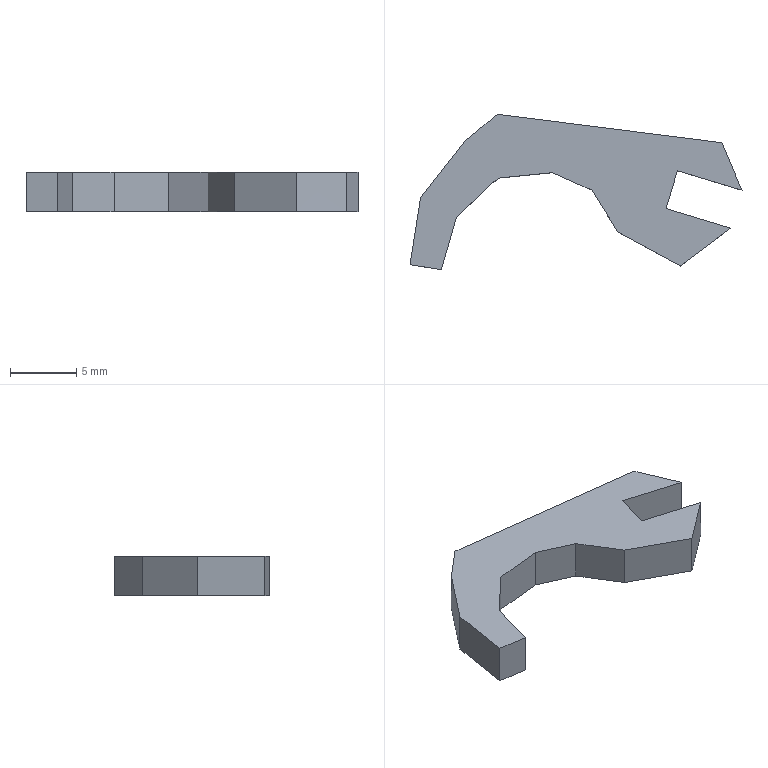Part | SolidWorks | features BaseBody 1 | 1 solid | 18 faces | box 25.116 x 11.758 x 3 mm | volume 409.356 mm3 | spline 12 | plane 6
STEP:
#1=CARTESIAN_POINT('',(49.749,1.825,-1.5));
#2=VERTEX_POINT('',#1);
#3=CARTESIAN_POINT('',(32.749,3.974,-1.5));
#4=VERTEX_POINT('',#3);
#5=CARTESIAN_POINT('',(49.749,1.825,-1.5));
#6=CARTESIAN_POINT('',(44.082,2.541,-1.5));
#7=CARTESIAN_POINT('',(38.416,3.258,-1.5));
#8=CARTESIAN_POINT('',(32.749,3.974,-1.5));
#9=B_SPLINE_CURVE_WITH_KNOTS('',3,(#5,#6,#7,#8),.UNSPECIFIED.,.F.,.F.,(4,4),(0.913,1.),.UNSPECIFIED.);
#10=EDGE_CURVE('',#2,#4,#9,.T.);
#11=ORIENTED_EDGE('',*,*,#10,.F.);
#12=CARTESIAN_POINT('',(51.278,-1.768,-1.5));
#13=VERTEX_POINT('',#12);
#14=CARTESIAN_POINT('',(51.278,-1.768,-1.5));
#15=DIRECTION('',(-0.3915,0.9202,0.));
#16=VECTOR('',#15,1000.);
#17=LINE('',#14,#16);
#18=EDGE_CURVE('',#13,#2,#17,.T.);
#19=ORIENTED_EDGE('',*,*,#18,.F.);
#20=CARTESIAN_POINT('',(46.394,-0.2969,-1.5));
#21=VERTEX_POINT('',#20);
#22=CARTESIAN_POINT('',(46.394,-0.2969,-1.5));
#23=DIRECTION('',(0.9575,-0.2885,0.));
#24=VECTOR('',#23,1000.);
#25=LINE('',#22,#24);
#26=EDGE_CURVE('',#21,#13,#25,.T.);
#27=ORIENTED_EDGE('',*,*,#26,.F.);
#28=CARTESIAN_POINT('',(45.529,-3.169,-1.5));
#29=VERTEX_POINT('',#28);
#30=CARTESIAN_POINT('',(45.529,-3.169,-1.5));
#31=DIRECTION('',(0.2885,0.9575,0.));
#32=VECTOR('',#31,1000.);
#33=LINE('',#30,#32);
#34=EDGE_CURVE('',#29,#21,#33,.T.);
#35=ORIENTED_EDGE('',*,*,#34,.F.);
#36=CARTESIAN_POINT('',(50.412,-4.641,-1.5));
#37=VERTEX_POINT('',#36);
#38=CARTESIAN_POINT('',(45.529,-3.169,-1.5));
#39=DIRECTION('',(-0.9575,0.2885,0.));
#40=VECTOR('',#39,1000.);
#41=LINE('',#38,#40);
#42=EDGE_CURVE('',#37,#29,#41,.T.);
#43=ORIENTED_EDGE('',*,*,#42,.F.);
#44=CARTESIAN_POINT('',(46.616,-7.504,-1.5));
#45=VERTEX_POINT('',#44);
#46=CARTESIAN_POINT('',(46.616,-7.504,-1.5));
#47=CARTESIAN_POINT('',(47.881,-6.548,-1.5));
#48=CARTESIAN_POINT('',(50.412,-4.641,-1.5));
#49=B_SPLINE_CURVE_WITH_KNOTS('',2,(#46,#47,#48),.UNSPECIFIED.,.F.,.F.,(3,3),(0.4348,0.4783),.UNSPECIFIED.);
#50=EDGE_CURVE('',#45,#37,#49,.T.);
#51=ORIENTED_EDGE('',*,*,#50,.F.);
#52=CARTESIAN_POINT('',(41.909,-4.958,-1.5));
#53=VERTEX_POINT('',#52);
#54=CARTESIAN_POINT('',(41.909,-4.958,-1.5));
#55=CARTESIAN_POINT('',(43.477,-5.807,-1.5));
#56=CARTESIAN_POINT('',(45.047,-6.655,-1.5));
#57=CARTESIAN_POINT('',(46.616,-7.504,-1.5));
#58=B_SPLINE_CURVE_WITH_KNOTS('',3,(#54,#55,#56,#57),.UNSPECIFIED.,.F.,.F.,(4,4),(0.3913,0.4348),.UNSPECIFIED.);
#59=EDGE_CURVE('',#53,#45,#58,.T.);
#60=ORIENTED_EDGE('',*,*,#59,.F.);
#61=CARTESIAN_POINT('',(39.937,-1.783,-1.5));
#62=VERTEX_POINT('',#61);
#63=CARTESIAN_POINT('',(39.937,-1.783,-1.5));
#64=CARTESIAN_POINT('',(40.594,-2.84,-1.5));
#65=CARTESIAN_POINT('',(41.252,-3.899,-1.5));
#66=CARTESIAN_POINT('',(41.909,-4.958,-1.5));
#67=B_SPLINE_CURVE_WITH_KNOTS('',3,(#63,#64,#65,#66),.UNSPECIFIED.,.F.,.F.,(4,4),(0.3478,0.3913),.UNSPECIFIED.);
#68=EDGE_CURVE('',#62,#53,#67,.T.);
#69=ORIENTED_EDGE('',*,*,#68,.F.);
#70=CARTESIAN_POINT('',(36.95,-0.4427,-1.5));
#71=VERTEX_POINT('',#70);
#72=CARTESIAN_POINT('',(36.95,-0.4427,-1.5));
#73=CARTESIAN_POINT('',(37.947,-0.8896,-1.5));
#74=CARTESIAN_POINT('',(38.941,-1.336,-1.5));
#75=CARTESIAN_POINT('',(39.937,-1.783,-1.5));
#76=B_SPLINE_CURVE_WITH_KNOTS('',3,(#72,#73,#74,#75),.UNSPECIFIED.,.F.,.F.,(4,4),(0.3043,0.3478),.UNSPECIFIED.);
#77=EDGE_CURVE('',#71,#62,#76,.T.);
#78=ORIENTED_EDGE('',*,*,#77,.F.);
#79=CARTESIAN_POINT('',(32.823,-0.8567,-1.5));
#80=VERTEX_POINT('',#79);
#81=CARTESIAN_POINT('',(32.823,-0.8567,-1.5));
#82=CARTESIAN_POINT('',(34.201,-0.7197,-1.5));
#83=CARTESIAN_POINT('',(35.575,-0.5811,-1.5));
#84=CARTESIAN_POINT('',(36.95,-0.4427,-1.5));
#85=B_SPLINE_CURVE_WITH_KNOTS('',3,(#81,#82,#83,#84),.UNSPECIFIED.,.F.,.F.,(4,4),(0.2609,0.3043),.UNSPECIFIED.);
#86=EDGE_CURVE('',#80,#71,#85,.T.);
#87=ORIENTED_EDGE('',*,*,#86,.F.);
#88=CARTESIAN_POINT('',(29.674,-3.825,-1.5));
#89=VERTEX_POINT('',#88);
#90=CARTESIAN_POINT('',(29.674,-3.825,-1.5));
#91=CARTESIAN_POINT('',(30.724,-2.835,-1.5));
#92=CARTESIAN_POINT('',(31.775,-1.846,-1.5));
#93=CARTESIAN_POINT('',(32.823,-0.8567,-1.5));
#94=B_SPLINE_CURVE_WITH_KNOTS('',3,(#90,#91,#92,#93),.UNSPECIFIED.,.F.,.F.,(4,4),(0.2174,0.2609),.UNSPECIFIED.);
#95=EDGE_CURVE('',#89,#80,#94,.T.);
#96=ORIENTED_EDGE('',*,*,#95,.F.);
#97=CARTESIAN_POINT('',(28.532,-7.783,-1.5));
#98=VERTEX_POINT('',#97);
#99=CARTESIAN_POINT('',(28.532,-7.783,-1.5));
#100=CARTESIAN_POINT('',(28.913,-6.463,-1.5));
#101=CARTESIAN_POINT('',(29.293,-5.143,-1.5));
#102=CARTESIAN_POINT('',(29.674,-3.825,-1.5));
#103=B_SPLINE_CURVE_WITH_KNOTS('',3,(#99,#100,#101,#102),.UNSPECIFIED.,.F.,.F.,(4,4),(0.1739,0.2174),.UNSPECIFIED.);
#104=EDGE_CURVE('',#98,#89,#103,.T.);
#105=ORIENTED_EDGE('',*,*,#104,.F.);
#106=CARTESIAN_POINT('',(26.162,-7.411,-1.5));
#107=VERTEX_POINT('',#106);
#108=CARTESIAN_POINT('',(26.162,-7.411,-1.5));
#109=CARTESIAN_POINT('',(26.952,-7.534,-1.5));
#110=CARTESIAN_POINT('',(27.742,-7.659,-1.5));
#111=CARTESIAN_POINT('',(28.532,-7.783,-1.5));
#112=B_SPLINE_CURVE_WITH_KNOTS('',3,(#108,#109,#110,#111),.UNSPECIFIED.,.F.,.F.,(4,4),(0.1304,0.1739),.UNSPECIFIED.);
#113=EDGE_CURVE('',#107,#98,#112,.T.);
#114=ORIENTED_EDGE('',*,*,#113,.F.);
#115=CARTESIAN_POINT('',(26.966,-2.331,-1.5));
#116=VERTEX_POINT('',#115);
#117=CARTESIAN_POINT('',(26.966,-2.331,-1.5));
#118=CARTESIAN_POINT('',(26.696,-4.024,-1.5));
#119=CARTESIAN_POINT('',(26.428,-5.716,-1.5));
#120=CARTESIAN_POINT('',(26.162,-7.411,-1.5));
#121=B_SPLINE_CURVE_WITH_KNOTS('',3,(#117,#118,#119,#120),.UNSPECIFIED.,.F.,.F.,(4,4),(0.08696,0.1304),.UNSPECIFIED.);
#122=EDGE_CURVE('',#116,#107,#121,.T.);
#123=ORIENTED_EDGE('',*,*,#122,.F.);
#124=CARTESIAN_POINT('',(30.236,1.845,-1.5));
#125=VERTEX_POINT('',#124);
#126=CARTESIAN_POINT('',(30.236,1.845,-1.5));
#127=CARTESIAN_POINT('',(29.145,0.4517,-1.5));
#128=CARTESIAN_POINT('',(28.055,-0.9382,-1.5));
#129=CARTESIAN_POINT('',(26.966,-2.331,-1.5));
#130=B_SPLINE_CURVE_WITH_KNOTS('',3,(#126,#127,#128,#129),.UNSPECIFIED.,.F.,.F.,(4,4),(0.04348,0.08696),.UNSPECIFIED.);
#131=EDGE_CURVE('',#125,#116,#130,.T.);
#132=ORIENTED_EDGE('',*,*,#131,.F.);
#133=CARTESIAN_POINT('',(32.749,3.974,-1.5));
#134=CARTESIAN_POINT('',(31.912,3.263,-1.5));
#135=CARTESIAN_POINT('',(31.073,2.553,-1.5));
#136=CARTESIAN_POINT('',(30.236,1.845,-1.5));
#137=B_SPLINE_CURVE_WITH_KNOTS('',3,(#133,#134,#135,#136),.UNSPECIFIED.,.F.,.F.,(4,4),(0.,0.04348),.UNSPECIFIED.);
#138=EDGE_CURVE('',#4,#125,#137,.T.);
#139=ORIENTED_EDGE('',*,*,#138,.F.);
#140=EDGE_LOOP('',(#11,#19,#27,#35,#43,#51,#60,#69,#78,#87,#96,#105,#114,#123,#132,#139));
#141=FACE_OUTER_BOUND('',#140,.T.);
#142=CARTESIAN_POINT('',(41.249,2.9,-1.5));
#143=DIRECTION('',(0.,0.,1.));
#144=DIRECTION('',(1.,0.,0.));
#145=AXIS2_PLACEMENT_3D('',#142,#143,#144);
#146=PLANE('',#145);
#147=ADVANCED_FACE('',(#141),#146,.F.);
#148=CARTESIAN_POINT('',(49.749,1.825,1.5));
#149=VERTEX_POINT('',#148);
#150=CARTESIAN_POINT('',(32.749,3.974,1.5));
#151=VERTEX_POINT('',#150);
#152=CARTESIAN_POINT('',(49.749,1.825,1.5));
#153=CARTESIAN_POINT('',(44.082,2.541,1.5));
#154=CARTESIAN_POINT('',(38.416,3.258,1.5));
#155=CARTESIAN_POINT('',(32.749,3.974,1.5));
#156=B_SPLINE_CURVE_WITH_KNOTS('',3,(#152,#153,#154,#155),.UNSPECIFIED.,.F.,.F.,(4,4),(0.913,1.),.UNSPECIFIED.);
#157=EDGE_CURVE('',#149,#151,#156,.T.);
#158=ORIENTED_EDGE('',*,*,#157,.T.);
#159=CARTESIAN_POINT('',(30.236,1.845,1.5));
#160=VERTEX_POINT('',#159);
#161=CARTESIAN_POINT('',(32.749,3.974,1.5));
#162=CARTESIAN_POINT('',(31.912,3.263,1.5));
#163=CARTESIAN_POINT('',(31.073,2.553,1.5));
#164=CARTESIAN_POINT('',(30.236,1.845,1.5));
#165=B_SPLINE_CURVE_WITH_KNOTS('',3,(#161,#162,#163,#164),.UNSPECIFIED.,.F.,.F.,(4,4),(0.,0.04348),.UNSPECIFIED.);
#166=EDGE_CURVE('',#151,#160,#165,.T.);
#167=ORIENTED_EDGE('',*,*,#166,.T.);
#168=CARTESIAN_POINT('',(26.966,-2.331,1.5));
#169=VERTEX_POINT('',#168);
#170=CARTESIAN_POINT('',(30.236,1.845,1.5));
#171=CARTESIAN_POINT('',(29.145,0.4517,1.5));
#172=CARTESIAN_POINT('',(28.055,-0.9382,1.5));
#173=CARTESIAN_POINT('',(26.966,-2.331,1.5));
#174=B_SPLINE_CURVE_WITH_KNOTS('',3,(#170,#171,#172,#173),.UNSPECIFIED.,.F.,.F.,(4,4),(0.04348,0.08696),.UNSPECIFIED.);
#175=EDGE_CURVE('',#160,#169,#174,.T.);
#176=ORIENTED_EDGE('',*,*,#175,.T.);
#177=CARTESIAN_POINT('',(26.162,-7.411,1.5));
#178=VERTEX_POINT('',#177);
#179=CARTESIAN_POINT('',(26.966,-2.331,1.5));
#180=CARTESIAN_POINT('',(26.696,-4.024,1.5));
#181=CARTESIAN_POINT('',(26.428,-5.716,1.5));
#182=CARTESIAN_POINT('',(26.162,-7.411,1.5));
#183=B_SPLINE_CURVE_WITH_KNOTS('',3,(#179,#180,#181,#182),.UNSPECIFIED.,.F.,.F.,(4,4),(0.08696,0.1304),.UNSPECIFIED.);
#184=EDGE_CURVE('',#169,#178,#183,.T.);
#185=ORIENTED_EDGE('',*,*,#184,.T.);
#186=CARTESIAN_POINT('',(28.532,-7.783,1.5));
#187=VERTEX_POINT('',#186);
#188=CARTESIAN_POINT('',(26.162,-7.411,1.5));
#189=CARTESIAN_POINT('',(26.952,-7.534,1.5));
#190=CARTESIAN_POINT('',(27.742,-7.659,1.5));
#191=CARTESIAN_POINT('',(28.532,-7.783,1.5));
#192=B_SPLINE_CURVE_WITH_KNOTS('',3,(#188,#189,#190,#191),.UNSPECIFIED.,.F.,.F.,(4,4),(0.1304,0.1739),.UNSPECIFIED.);
#193=EDGE_CURVE('',#178,#187,#192,.T.);
#194=ORIENTED_EDGE('',*,*,#193,.T.);
#195=CARTESIAN_POINT('',(29.674,-3.825,1.5));
#196=VERTEX_POINT('',#195);
#197=CARTESIAN_POINT('',(28.532,-7.783,1.5));
#198=CARTESIAN_POINT('',(28.913,-6.463,1.5));
#199=CARTESIAN_POINT('',(29.293,-5.143,1.5));
#200=CARTESIAN_POINT('',(29.674,-3.825,1.5));
#201=B_SPLINE_CURVE_WITH_KNOTS('',3,(#197,#198,#199,#200),.UNSPECIFIED.,.F.,.F.,(4,4),(0.1739,0.2174),.UNSPECIFIED.);
#202=EDGE_CURVE('',#187,#196,#201,.T.);
#203=ORIENTED_EDGE('',*,*,#202,.T.);
#204=CARTESIAN_POINT('',(32.823,-0.8567,1.5));
#205=VERTEX_POINT('',#204);
#206=CARTESIAN_POINT('',(29.674,-3.825,1.5));
#207=CARTESIAN_POINT('',(30.724,-2.835,1.5));
#208=CARTESIAN_POINT('',(31.775,-1.846,1.5));
#209=CARTESIAN_POINT('',(32.823,-0.8567,1.5));
#210=B_SPLINE_CURVE_WITH_KNOTS('',3,(#206,#207,#208,#209),.UNSPECIFIED.,.F.,.F.,(4,4),(0.2174,0.2609),.UNSPECIFIED.);
#211=EDGE_CURVE('',#196,#205,#210,.T.);
#212=ORIENTED_EDGE('',*,*,#211,.T.);
#213=CARTESIAN_POINT('',(36.95,-0.4427,1.5));
#214=VERTEX_POINT('',#213);
#215=CARTESIAN_POINT('',(32.823,-0.8567,1.5));
#216=CARTESIAN_POINT('',(34.201,-0.7197,1.5));
#217=CARTESIAN_POINT('',(35.575,-0.5811,1.5));
#218=CARTESIAN_POINT('',(36.95,-0.4427,1.5));
#219=B_SPLINE_CURVE_WITH_KNOTS('',3,(#215,#216,#217,#218),.UNSPECIFIED.,.F.,.F.,(4,4),(0.2609,0.3043),.UNSPECIFIED.);
#220=EDGE_CURVE('',#205,#214,#219,.T.);
#221=ORIENTED_EDGE('',*,*,#220,.T.);
#222=CARTESIAN_POINT('',(39.937,-1.783,1.5));
#223=VERTEX_POINT('',#222);
#224=CARTESIAN_POINT('',(36.95,-0.4427,1.5));
#225=CARTESIAN_POINT('',(37.947,-0.8896,1.5));
#226=CARTESIAN_POINT('',(38.941,-1.336,1.5));
#227=CARTESIAN_POINT('',(39.937,-1.783,1.5));
#228=B_SPLINE_CURVE_WITH_KNOTS('',3,(#224,#225,#226,#227),.UNSPECIFIED.,.F.,.F.,(4,4),(0.3043,0.3478),.UNSPECIFIED.);
#229=EDGE_CURVE('',#214,#223,#228,.T.);
#230=ORIENTED_EDGE('',*,*,#229,.T.);
#231=CARTESIAN_POINT('',(41.909,-4.958,1.5));
#232=VERTEX_POINT('',#231);
#233=CARTESIAN_POINT('',(39.937,-1.783,1.5));
#234=CARTESIAN_POINT('',(40.594,-2.84,1.5));
#235=CARTESIAN_POINT('',(41.252,-3.899,1.5));
#236=CARTESIAN_POINT('',(41.909,-4.958,1.5));
#237=B_SPLINE_CURVE_WITH_KNOTS('',3,(#233,#234,#235,#236),.UNSPECIFIED.,.F.,.F.,(4,4),(0.3478,0.3913),.UNSPECIFIED.);
#238=EDGE_CURVE('',#223,#232,#237,.T.);
#239=ORIENTED_EDGE('',*,*,#238,.T.);
#240=CARTESIAN_POINT('',(46.616,-7.504,1.5));
#241=VERTEX_POINT('',#240);
#242=CARTESIAN_POINT('',(41.909,-4.958,1.5));
#243=CARTESIAN_POINT('',(43.477,-5.807,1.5));
#244=CARTESIAN_POINT('',(45.047,-6.655,1.5));
#245=CARTESIAN_POINT('',(46.616,-7.504,1.5));
#246=B_SPLINE_CURVE_WITH_KNOTS('',3,(#242,#243,#244,#245),.UNSPECIFIED.,.F.,.F.,(4,4),(0.3913,0.4348),.UNSPECIFIED.);
#247=EDGE_CURVE('',#232,#241,#246,.T.);
#248=ORIENTED_EDGE('',*,*,#247,.T.);
#249=CARTESIAN_POINT('',(50.412,-4.641,1.5));
#250=VERTEX_POINT('',#249);
#251=CARTESIAN_POINT('',(46.616,-7.504,1.5));
#252=CARTESIAN_POINT('',(47.881,-6.548,1.5));
#253=CARTESIAN_POINT('',(50.412,-4.641,1.5));
#254=B_SPLINE_CURVE_WITH_KNOTS('',2,(#251,#252,#253),.UNSPECIFIED.,.F.,.F.,(3,3),(0.4348,0.4783),.UNSPECIFIED.);
#255=EDGE_CURVE('',#241,#250,#254,.T.);
#256=ORIENTED_EDGE('',*,*,#255,.T.);
#257=CARTESIAN_POINT('',(45.529,-3.169,1.5));
#258=VERTEX_POINT('',#257);
#259=CARTESIAN_POINT('',(45.529,-3.169,1.5));
#260=DIRECTION('',(-0.9575,0.2885,0.));
#261=VECTOR('',#260,1000.);
#262=LINE('',#259,#261);
#263=EDGE_CURVE('',#250,#258,#262,.T.);
#264=ORIENTED_EDGE('',*,*,#263,.T.);
#265=CARTESIAN_POINT('',(46.394,-0.2969,1.5));
#266=VERTEX_POINT('',#265);
#267=CARTESIAN_POINT('',(45.529,-3.169,1.5));
#268=DIRECTION('',(0.2885,0.9575,0.));
#269=VECTOR('',#268,1000.);
#270=LINE('',#267,#269);
#271=EDGE_CURVE('',#258,#266,#270,.T.);
#272=ORIENTED_EDGE('',*,*,#271,.T.);
#273=CARTESIAN_POINT('',(51.278,-1.768,1.5));
#274=VERTEX_POINT('',#273);
#275=CARTESIAN_POINT('',(46.394,-0.2969,1.5));
#276=DIRECTION('',(0.9575,-0.2885,0.));
#277=VECTOR('',#276,1000.);
#278=LINE('',#275,#277);
#279=EDGE_CURVE('',#266,#274,#278,.T.);
#280=ORIENTED_EDGE('',*,*,#279,.T.);
#281=CARTESIAN_POINT('',(51.278,-1.768,1.5));
#282=DIRECTION('',(-0.3915,0.9202,0.));
#283=VECTOR('',#282,1000.);
#284=LINE('',#281,#283);
#285=EDGE_CURVE('',#274,#149,#284,.T.);
#286=ORIENTED_EDGE('',*,*,#285,.T.);
#287=EDGE_LOOP('',(#158,#167,#176,#185,#194,#203,#212,#221,#230,#239,#248,#256,#264,#272,#280,#286));
#288=FACE_OUTER_BOUND('',#287,.T.);
#289=CARTESIAN_POINT('',(41.249,2.9,1.5));
#290=DIRECTION('',(0.,0.,1.));
#291=DIRECTION('',(1.,0.,0.));
#292=AXIS2_PLACEMENT_3D('',#289,#290,#291);
#293=PLANE('',#292);
#294=ADVANCED_FACE('',(#288),#293,.T.);
#295=ORIENTED_EDGE('',*,*,#18,.T.);
#296=CARTESIAN_POINT('',(49.749,1.825,1.5));
#297=DIRECTION('',(0.,0.,-1.));
#298=VECTOR('',#297,1000.);
#299=LINE('',#296,#298);
#300=EDGE_CURVE('',#149,#2,#299,.T.);
#301=ORIENTED_EDGE('',*,*,#300,.F.);
#302=ORIENTED_EDGE('',*,*,#285,.F.);
#303=CARTESIAN_POINT('',(51.278,-1.768,1.5));
#304=DIRECTION('',(0.,0.,-1.));
#305=VECTOR('',#304,1000.);
#306=LINE('',#303,#305);
#307=EDGE_CURVE('',#274,#13,#306,.T.);
#308=ORIENTED_EDGE('',*,*,#307,.T.);
#309=EDGE_LOOP('',(#295,#301,#302,#308));
#310=FACE_OUTER_BOUND('',#309,.T.);
#311=CARTESIAN_POINT('',(51.278,-1.768,1.5));
#312=DIRECTION('',(-0.9202,-0.3915,0.));
#313=DIRECTION('',(-0.3915,0.9202,0.));
#314=AXIS2_PLACEMENT_3D('',#311,#312,#313);
#315=PLANE('',#314);
#316=ADVANCED_FACE('',(#310),#315,.F.);
#317=ORIENTED_EDGE('',*,*,#26,.T.);
#318=ORIENTED_EDGE('',*,*,#307,.F.);
#319=ORIENTED_EDGE('',*,*,#279,.F.);
#320=CARTESIAN_POINT('',(46.394,-0.2969,1.5));
#321=DIRECTION('',(0.,0.,-1.));
#322=VECTOR('',#321,1000.);
#323=LINE('',#320,#322);
#324=EDGE_CURVE('',#266,#21,#323,.T.);
#325=ORIENTED_EDGE('',*,*,#324,.T.);
#326=EDGE_LOOP('',(#317,#318,#319,#325));
#327=FACE_OUTER_BOUND('',#326,.T.);
#328=CARTESIAN_POINT('',(46.394,-0.2969,1.5));
#329=DIRECTION('',(0.2885,0.9575,0.));
#330=DIRECTION('',(0.,0.,-1.));
#331=AXIS2_PLACEMENT_3D('',#328,#329,#330);
#332=PLANE('',#331);
#333=ADVANCED_FACE('',(#327),#332,.F.);
#334=ORIENTED_EDGE('',*,*,#34,.T.);
#335=ORIENTED_EDGE('',*,*,#324,.F.);
#336=ORIENTED_EDGE('',*,*,#271,.F.);
#337=CARTESIAN_POINT('',(45.529,-3.169,1.5));
#338=DIRECTION('',(0.,0.,-1.));
#339=VECTOR('',#338,1000.);
#340=LINE('',#337,#339);
#341=EDGE_CURVE('',#258,#29,#340,.T.);
#342=ORIENTED_EDGE('',*,*,#341,.T.);
#343=EDGE_LOOP('',(#334,#335,#336,#342));
#344=FACE_OUTER_BOUND('',#343,.T.);
#345=CARTESIAN_POINT('',(45.529,-3.169,1.5));
#346=DIRECTION('',(-0.9575,0.2885,0.));
#347=DIRECTION('',(0.,0.,1.));
#348=AXIS2_PLACEMENT_3D('',#345,#346,#347);
#349=PLANE('',#348);
#350=ADVANCED_FACE('',(#344),#349,.F.);
#351=ORIENTED_EDGE('',*,*,#42,.T.);
#352=ORIENTED_EDGE('',*,*,#341,.F.);
#353=ORIENTED_EDGE('',*,*,#263,.F.);
#354=CARTESIAN_POINT('',(50.412,-4.641,1.5));
#355=DIRECTION('',(0.,0.,-1.));
#356=VECTOR('',#355,1000.);
#357=LINE('',#354,#356);
#358=EDGE_CURVE('',#250,#37,#357,.T.);
#359=ORIENTED_EDGE('',*,*,#358,.T.);
#360=EDGE_LOOP('',(#351,#352,#353,#359));
#361=FACE_OUTER_BOUND('',#360,.T.);
#362=CARTESIAN_POINT('',(45.529,-3.169,1.5));
#363=DIRECTION('',(-0.2885,-0.9575,0.));
#364=DIRECTION('',(-0.9575,0.2885,0.));
#365=AXIS2_PLACEMENT_3D('',#362,#363,#364);
#366=PLANE('',#365);
#367=ADVANCED_FACE('',(#361),#366,.F.);
#368=ORIENTED_EDGE('',*,*,#50,.T.);
#369=ORIENTED_EDGE('',*,*,#358,.F.);
#370=ORIENTED_EDGE('',*,*,#255,.F.);
#371=CARTESIAN_POINT('',(46.616,-7.504,1.5));
#372=DIRECTION('',(0.,0.,-1.));
#373=VECTOR('',#372,1000.);
#374=LINE('',#371,#373);
#375=EDGE_CURVE('',#241,#45,#374,.T.);
#376=ORIENTED_EDGE('',*,*,#375,.T.);
#377=EDGE_LOOP('',(#368,#369,#370,#376));
#378=FACE_OUTER_BOUND('',#377,.T.);
#379=CARTESIAN_POINT('',(46.616,-7.504,1.5));
#380=CARTESIAN_POINT('',(46.616,-7.504,-1.5));
#381=CARTESIAN_POINT('',(47.881,-6.548,1.5));
#382=CARTESIAN_POINT('',(47.881,-6.548,-1.5));
#383=CARTESIAN_POINT('',(50.412,-4.641,1.5));
#384=CARTESIAN_POINT('',(50.412,-4.641,-1.5));
#385=B_SPLINE_SURFACE_WITH_KNOTS('',2,1,((#379,#380),(#381,#382),(#383,#384)),.UNSPECIFIED.,.F.,.F.,.F.,(3,3),(2,2),(0.4348,0.4783),(0.,1.),.UNSPECIFIED.);
#386=ADVANCED_FACE('',(#378),#385,.F.);
#387=ORIENTED_EDGE('',*,*,#59,.T.);
#388=ORIENTED_EDGE('',*,*,#375,.F.);
#389=ORIENTED_EDGE('',*,*,#247,.F.);
#390=CARTESIAN_POINT('',(41.909,-4.958,1.5));
#391=DIRECTION('',(0.,0.,-1.));
#392=VECTOR('',#391,1000.);
#393=LINE('',#390,#392);
#394=EDGE_CURVE('',#232,#53,#393,.T.);
#395=ORIENTED_EDGE('',*,*,#394,.T.);
#396=EDGE_LOOP('',(#387,#388,#389,#395));
#397=FACE_OUTER_BOUND('',#396,.T.);
#398=CARTESIAN_POINT('',(41.909,-4.958,1.5));
#399=CARTESIAN_POINT('',(41.909,-4.958,-1.5));
#400=CARTESIAN_POINT('',(43.477,-5.807,1.5));
#401=CARTESIAN_POINT('',(43.477,-5.807,-1.5));
#402=CARTESIAN_POINT('',(45.047,-6.655,1.5));
#403=CARTESIAN_POINT('',(45.047,-6.655,-1.5));
#404=CARTESIAN_POINT('',(46.616,-7.504,1.5));
#405=CARTESIAN_POINT('',(46.616,-7.504,-1.5));
#406=B_SPLINE_SURFACE_WITH_KNOTS('',3,1,((#398,#399),(#400,#401),(#402,#403),(#404,#405)),.UNSPECIFIED.,.F.,.F.,.F.,(4,4),(2,2),(0.3913,0.4348),(0.,1.),.UNSPECIFIED.);
#407=ADVANCED_FACE('',(#397),#406,.F.);
#408=ORIENTED_EDGE('',*,*,#68,.T.);
#409=ORIENTED_EDGE('',*,*,#394,.F.);
#410=ORIENTED_EDGE('',*,*,#238,.F.);
#411=CARTESIAN_POINT('',(39.937,-1.783,1.5));
#412=DIRECTION('',(0.,0.,-1.));
#413=VECTOR('',#412,1000.);
#414=LINE('',#411,#413);
#415=EDGE_CURVE('',#223,#62,#414,.T.);
#416=ORIENTED_EDGE('',*,*,#415,.T.);
#417=EDGE_LOOP('',(#408,#409,#410,#416));
#418=FACE_OUTER_BOUND('',#417,.T.);
#419=CARTESIAN_POINT('',(39.937,-1.783,1.5));
#420=CARTESIAN_POINT('',(39.937,-1.783,-1.5));
#421=CARTESIAN_POINT('',(40.594,-2.84,1.5));
#422=CARTESIAN_POINT('',(40.594,-2.84,-1.5));
#423=CARTESIAN_POINT('',(41.252,-3.899,1.5));
#424=CARTESIAN_POINT('',(41.252,-3.899,-1.5));
#425=CARTESIAN_POINT('',(41.909,-4.958,1.5));
#426=CARTESIAN_POINT('',(41.909,-4.958,-1.5));
#427=B_SPLINE_SURFACE_WITH_KNOTS('',3,1,((#419,#420),(#421,#422),(#423,#424),(#425,#426)),.UNSPECIFIED.,.F.,.F.,.F.,(4,4),(2,2),(0.3478,0.3913),(0.,1.),.UNSPECIFIED.);
#428=ADVANCED_FACE('',(#418),#427,.F.);
#429=ORIENTED_EDGE('',*,*,#77,.T.);
#430=ORIENTED_EDGE('',*,*,#415,.F.);
#431=ORIENTED_EDGE('',*,*,#229,.F.);
#432=CARTESIAN_POINT('',(36.95,-0.4427,1.5));
#433=DIRECTION('',(0.,0.,-1.));
#434=VECTOR('',#433,1000.);
#435=LINE('',#432,#434);
#436=EDGE_CURVE('',#214,#71,#435,.T.);
#437=ORIENTED_EDGE('',*,*,#436,.T.);
#438=EDGE_LOOP('',(#429,#430,#431,#437));
#439=FACE_OUTER_BOUND('',#438,.T.);
#440=CARTESIAN_POINT('',(36.95,-0.4427,1.5));
#441=CARTESIAN_POINT('',(36.95,-0.4427,-1.5));
#442=CARTESIAN_POINT('',(37.947,-0.8896,1.5));
#443=CARTESIAN_POINT('',(37.947,-0.8896,-1.5));
#444=CARTESIAN_POINT('',(38.941,-1.336,1.5));
#445=CARTESIAN_POINT('',(38.941,-1.336,-1.5));
#446=CARTESIAN_POINT('',(39.937,-1.783,1.5));
#447=CARTESIAN_POINT('',(39.937,-1.783,-1.5));
#448=B_SPLINE_SURFACE_WITH_KNOTS('',3,1,((#440,#441),(#442,#443),(#444,#445),(#446,#447)),.UNSPECIFIED.,.F.,.F.,.F.,(4,4),(2,2),(0.3043,0.3478),(0.,1.),.UNSPECIFIED.);
#449=ADVANCED_FACE('',(#439),#448,.F.);
#450=ORIENTED_EDGE('',*,*,#86,.T.);
#451=ORIENTED_EDGE('',*,*,#436,.F.);
#452=ORIENTED_EDGE('',*,*,#220,.F.);
#453=CARTESIAN_POINT('',(32.823,-0.8567,1.5));
#454=DIRECTION('',(0.,0.,-1.));
#455=VECTOR('',#454,1000.);
#456=LINE('',#453,#455);
#457=EDGE_CURVE('',#205,#80,#456,.T.);
#458=ORIENTED_EDGE('',*,*,#457,.T.);
#459=EDGE_LOOP('',(#450,#451,#452,#458));
#460=FACE_OUTER_BOUND('',#459,.T.);
#461=CARTESIAN_POINT('',(32.823,-0.8567,1.5));
#462=CARTESIAN_POINT('',(32.823,-0.8567,-1.5));
#463=CARTESIAN_POINT('',(34.201,-0.7197,1.5));
#464=CARTESIAN_POINT('',(34.201,-0.7197,-1.5));
#465=CARTESIAN_POINT('',(35.575,-0.5811,1.5));
#466=CARTESIAN_POINT('',(35.575,-0.5811,-1.5));
#467=CARTESIAN_POINT('',(36.95,-0.4427,1.5));
#468=CARTESIAN_POINT('',(36.95,-0.4427,-1.5));
#469=B_SPLINE_SURFACE_WITH_KNOTS('',3,1,((#461,#462),(#463,#464),(#465,#466),(#467,#468)),.UNSPECIFIED.,.F.,.F.,.F.,(4,4),(2,2),(0.2609,0.3043),(0.,1.),.UNSPECIFIED.);
#470=ADVANCED_FACE('',(#460),#469,.F.);
#471=ORIENTED_EDGE('',*,*,#95,.T.);
#472=ORIENTED_EDGE('',*,*,#457,.F.);
#473=ORIENTED_EDGE('',*,*,#211,.F.);
#474=CARTESIAN_POINT('',(29.674,-3.825,1.5));
#475=DIRECTION('',(0.,0.,-1.));
#476=VECTOR('',#475,1000.);
#477=LINE('',#474,#476);
#478=EDGE_CURVE('',#196,#89,#477,.T.);
#479=ORIENTED_EDGE('',*,*,#478,.T.);
#480=EDGE_LOOP('',(#471,#472,#473,#479));
#481=FACE_OUTER_BOUND('',#480,.T.);
#482=CARTESIAN_POINT('',(29.674,-3.825,1.5));
#483=CARTESIAN_POINT('',(29.674,-3.825,-1.5));
#484=CARTESIAN_POINT('',(30.724,-2.835,1.5));
#485=CARTESIAN_POINT('',(30.724,-2.835,-1.5));
#486=CARTESIAN_POINT('',(31.775,-1.846,1.5));
#487=CARTESIAN_POINT('',(31.775,-1.846,-1.5));
#488=CARTESIAN_POINT('',(32.823,-0.8567,1.5));
#489=CARTESIAN_POINT('',(32.823,-0.8567,-1.5));
#490=B_SPLINE_SURFACE_WITH_KNOTS('',3,1,((#482,#483),(#484,#485),(#486,#487),(#488,#489)),.UNSPECIFIED.,.F.,.F.,.F.,(4,4),(2,2),(0.2174,0.2609),(0.,1.),.UNSPECIFIED.);
#491=ADVANCED_FACE('',(#481),#490,.F.);
#492=ORIENTED_EDGE('',*,*,#104,.T.);
#493=ORIENTED_EDGE('',*,*,#478,.F.);
#494=ORIENTED_EDGE('',*,*,#202,.F.);
#495=CARTESIAN_POINT('',(28.532,-7.783,1.5));
#496=DIRECTION('',(0.,0.,-1.));
#497=VECTOR('',#496,1000.);
#498=LINE('',#495,#497);
#499=EDGE_CURVE('',#187,#98,#498,.T.);
#500=ORIENTED_EDGE('',*,*,#499,.T.);
#501=EDGE_LOOP('',(#492,#493,#494,#500));
#502=FACE_OUTER_BOUND('',#501,.T.);
#503=CARTESIAN_POINT('',(28.532,-7.783,1.5));
#504=CARTESIAN_POINT('',(28.532,-7.783,-1.5));
#505=CARTESIAN_POINT('',(28.913,-6.463,1.5));
#506=CARTESIAN_POINT('',(28.913,-6.463,-1.5));
#507=CARTESIAN_POINT('',(29.293,-5.143,1.5));
#508=CARTESIAN_POINT('',(29.293,-5.143,-1.5));
#509=CARTESIAN_POINT('',(29.674,-3.825,1.5));
#510=CARTESIAN_POINT('',(29.674,-3.825,-1.5));
#511=B_SPLINE_SURFACE_WITH_KNOTS('',3,1,((#503,#504),(#505,#506),(#507,#508),(#509,#510)),.UNSPECIFIED.,.F.,.F.,.F.,(4,4),(2,2),(0.1739,0.2174),(0.,1.),.UNSPECIFIED.);
#512=ADVANCED_FACE('',(#502),#511,.F.);
#513=ORIENTED_EDGE('',*,*,#113,.T.);
#514=ORIENTED_EDGE('',*,*,#499,.F.);
#515=ORIENTED_EDGE('',*,*,#193,.F.);
#516=CARTESIAN_POINT('',(26.162,-7.411,1.5));
#517=DIRECTION('',(0.,0.,-1.));
#518=VECTOR('',#517,1000.);
#519=LINE('',#516,#518);
#520=EDGE_CURVE('',#178,#107,#519,.T.);
#521=ORIENTED_EDGE('',*,*,#520,.T.);
#522=EDGE_LOOP('',(#513,#514,#515,#521));
#523=FACE_OUTER_BOUND('',#522,.T.);
#524=CARTESIAN_POINT('',(26.162,-7.411,1.5));
#525=CARTESIAN_POINT('',(26.162,-7.411,-1.5));
#526=CARTESIAN_POINT('',(26.952,-7.534,1.5));
#527=CARTESIAN_POINT('',(26.952,-7.534,-1.5));
#528=CARTESIAN_POINT('',(27.742,-7.659,1.5));
#529=CARTESIAN_POINT('',(27.742,-7.659,-1.5));
#530=CARTESIAN_POINT('',(28.532,-7.783,1.5));
#531=CARTESIAN_POINT('',(28.532,-7.783,-1.5));
#532=B_SPLINE_SURFACE_WITH_KNOTS('',3,1,((#524,#525),(#526,#527),(#528,#529),(#530,#531)),.UNSPECIFIED.,.F.,.F.,.F.,(4,4),(2,2),(0.1304,0.1739),(0.,1.),.UNSPECIFIED.);
#533=ADVANCED_FACE('',(#523),#532,.F.);
#534=ORIENTED_EDGE('',*,*,#122,.T.);
#535=ORIENTED_EDGE('',*,*,#520,.F.);
#536=ORIENTED_EDGE('',*,*,#184,.F.);
#537=CARTESIAN_POINT('',(26.966,-2.331,1.5));
#538=DIRECTION('',(0.,0.,-1.));
#539=VECTOR('',#538,1000.);
#540=LINE('',#537,#539);
#541=EDGE_CURVE('',#169,#116,#540,.T.);
#542=ORIENTED_EDGE('',*,*,#541,.T.);
#543=EDGE_LOOP('',(#534,#535,#536,#542));
#544=FACE_OUTER_BOUND('',#543,.T.);
#545=CARTESIAN_POINT('',(26.966,-2.331,1.5));
#546=CARTESIAN_POINT('',(26.966,-2.331,-1.5));
#547=CARTESIAN_POINT('',(26.696,-4.024,1.5));
#548=CARTESIAN_POINT('',(26.696,-4.024,-1.5));
#549=CARTESIAN_POINT('',(26.428,-5.716,1.5));
#550=CARTESIAN_POINT('',(26.428,-5.716,-1.5));
#551=CARTESIAN_POINT('',(26.162,-7.411,1.5));
#552=CARTESIAN_POINT('',(26.162,-7.411,-1.5));
#553=B_SPLINE_SURFACE_WITH_KNOTS('',3,1,((#545,#546),(#547,#548),(#549,#550),(#551,#552)),.UNSPECIFIED.,.F.,.F.,.F.,(4,4),(2,2),(0.08696,0.1304),(0.,1.),.UNSPECIFIED.);
#554=ADVANCED_FACE('',(#544),#553,.F.);
#555=ORIENTED_EDGE('',*,*,#131,.T.);
#556=ORIENTED_EDGE('',*,*,#541,.F.);
#557=ORIENTED_EDGE('',*,*,#175,.F.);
#558=CARTESIAN_POINT('',(30.236,1.845,1.5));
#559=DIRECTION('',(0.,0.,-1.));
#560=VECTOR('',#559,1000.);
#561=LINE('',#558,#560);
#562=EDGE_CURVE('',#160,#125,#561,.T.);
#563=ORIENTED_EDGE('',*,*,#562,.T.);
#564=EDGE_LOOP('',(#555,#556,#557,#563));
#565=FACE_OUTER_BOUND('',#564,.T.);
#566=CARTESIAN_POINT('',(30.236,1.845,1.5));
#567=CARTESIAN_POINT('',(30.236,1.845,-1.5));
#568=CARTESIAN_POINT('',(29.145,0.4517,1.5));
#569=CARTESIAN_POINT('',(29.145,0.4517,-1.5));
#570=CARTESIAN_POINT('',(28.055,-0.9382,1.5));
#571=CARTESIAN_POINT('',(28.055,-0.9382,-1.5));
#572=CARTESIAN_POINT('',(26.966,-2.331,1.5));
#573=CARTESIAN_POINT('',(26.966,-2.331,-1.5));
#574=B_SPLINE_SURFACE_WITH_KNOTS('',3,1,((#566,#567),(#568,#569),(#570,#571),(#572,#573)),.UNSPECIFIED.,.F.,.F.,.F.,(4,4),(2,2),(0.04348,0.08696),(0.,1.),.UNSPECIFIED.);
#575=ADVANCED_FACE('',(#565),#574,.F.);
#576=ORIENTED_EDGE('',*,*,#138,.T.);
#577=ORIENTED_EDGE('',*,*,#562,.F.);
#578=ORIENTED_EDGE('',*,*,#166,.F.);
#579=CARTESIAN_POINT('',(32.749,3.974,1.5));
#580=DIRECTION('',(0.,0.,-1.));
#581=VECTOR('',#580,1000.);
#582=LINE('',#579,#581);
#583=EDGE_CURVE('',#151,#4,#582,.T.);
#584=ORIENTED_EDGE('',*,*,#583,.T.);
#585=EDGE_LOOP('',(#576,#577,#578,#584));
#586=FACE_OUTER_BOUND('',#585,.T.);
#587=CARTESIAN_POINT('',(32.749,3.974,1.5));
#588=CARTESIAN_POINT('',(32.749,3.974,-1.5));
#589=CARTESIAN_POINT('',(31.912,3.263,1.5));
#590=CARTESIAN_POINT('',(31.912,3.263,-1.5));
#591=CARTESIAN_POINT('',(31.073,2.553,1.5));
#592=CARTESIAN_POINT('',(31.073,2.553,-1.5));
#593=CARTESIAN_POINT('',(30.236,1.845,1.5));
#594=CARTESIAN_POINT('',(30.236,1.845,-1.5));
#595=B_SPLINE_SURFACE_WITH_KNOTS('',3,1,((#587,#588),(#589,#590),(#591,#592),(#593,#594)),.UNSPECIFIED.,.F.,.F.,.F.,(4,4),(2,2),(0.,0.04348),(0.,1.),.UNSPECIFIED.);
#596=ADVANCED_FACE('',(#586),#595,.F.);
#597=ORIENTED_EDGE('',*,*,#10,.T.);
#598=ORIENTED_EDGE('',*,*,#583,.F.);
#599=ORIENTED_EDGE('',*,*,#157,.F.);
#600=ORIENTED_EDGE('',*,*,#300,.T.);
#601=EDGE_LOOP('',(#597,#598,#599,#600));
#602=FACE_OUTER_BOUND('',#601,.T.);
#603=CARTESIAN_POINT('',(49.749,1.825,1.5));
#604=CARTESIAN_POINT('',(49.749,1.825,-1.5));
#605=CARTESIAN_POINT('',(44.082,2.541,1.5));
#606=CARTESIAN_POINT('',(44.082,2.541,-1.5));
#607=CARTESIAN_POINT('',(38.416,3.258,1.5));
#608=CARTESIAN_POINT('',(38.416,3.258,-1.5));
#609=CARTESIAN_POINT('',(32.749,3.974,1.5));
#610=CARTESIAN_POINT('',(32.749,3.974,-1.5));
#611=B_SPLINE_SURFACE_WITH_KNOTS('',3,1,((#603,#604),(#605,#606),(#607,#608),(#609,#610)),.UNSPECIFIED.,.F.,.F.,.F.,(4,4),(2,2),(0.913,1.),(0.,1.),.UNSPECIFIED.);
#612=ADVANCED_FACE('',(#602),#611,.F.);
#613=CLOSED_SHELL('',(#147,#294,#316,#333,#350,#367,#386,#407,#428,#449,#470,#491,#512,#533,#554,#575,#596,#612));
#614=MANIFOLD_SOLID_BREP('',#613);
#615=CARTESIAN_POINT('',(0.,0.,0.));
#616=DIRECTION('',(0.,0.,1.));
#617=DIRECTION('',(1.,0.,0.));
#618=AXIS2_PLACEMENT_3D('',#615,#616,#617);
#619=(LENGTH_UNIT()NAMED_UNIT(*)SI_UNIT(.MILLI.,.METRE.));
#620=UNCERTAINTY_MEASURE_WITH_UNIT(LENGTH_MEASURE(0.00001),#619,'','');
#621=(NAMED_UNIT(*)PLANE_ANGLE_UNIT()SI_UNIT($,.RADIAN.));
#622=(NAMED_UNIT(*)SI_UNIT($,.STERADIAN.)SOLID_ANGLE_UNIT());
#623=(GEOMETRIC_REPRESENTATION_CONTEXT(3)GLOBAL_UNCERTAINTY_ASSIGNED_CONTEXT((#620))GLOBAL_UNIT_ASSIGNED_CONTEXT((#619,#621,#622))REPRESENTATION_CONTEXT('',''));
#624=ADVANCED_BREP_SHAPE_REPRESENTATION('',(#614,#618),#623);